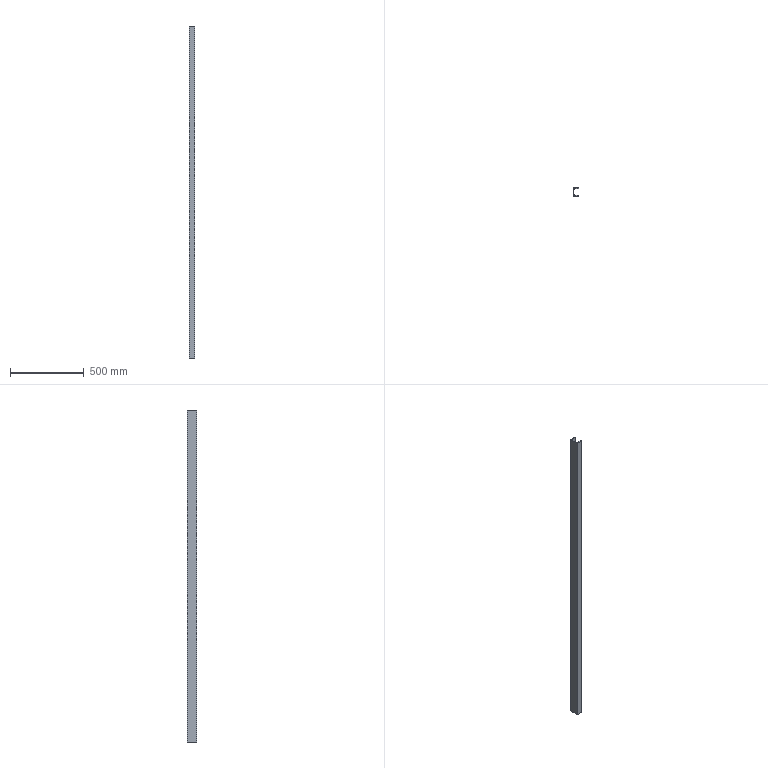Part | STEP file | 750038459 | 1 solid | 14 faces | box 40 x 63 x 2248 mm | volume 1898587 mm3 | plane 10 | cylinder 4 | commonest cylinder face diameters 7.6 x2 15 x2
STEP:
#1=CARTESIAN_POINT('',(0.,0.,2248.));
#2=VERTEX_POINT('',#1);
#3=CARTESIAN_POINT('',(0.,0.,0.));
#4=VERTEX_POINT('',#3);
#5=CARTESIAN_POINT('',(0.,0.,2248.));
#6=DIRECTION('',(0.,0.,-1.));
#7=VECTOR('',#6,1000.);
#8=LINE('',#5,#7);
#9=EDGE_CURVE('',#2,#4,#8,.T.);
#10=ORIENTED_EDGE('',*,*,#9,.F.);
#11=CARTESIAN_POINT('',(0.,63.,2248.));
#12=VERTEX_POINT('',#11);
#13=CARTESIAN_POINT('',(0.,63.,2248.));
#14=DIRECTION('',(0.,-1.,0.));
#15=VECTOR('',#14,1000.);
#16=LINE('',#13,#15);
#17=EDGE_CURVE('',#12,#2,#16,.T.);
#18=ORIENTED_EDGE('',*,*,#17,.F.);
#19=CARTESIAN_POINT('',(0.,63.,0.));
#20=VERTEX_POINT('',#19);
#21=CARTESIAN_POINT('',(0.,63.,2248.));
#22=DIRECTION('',(0.,0.,1.));
#23=VECTOR('',#22,1000.);
#24=LINE('',#21,#23);
#25=EDGE_CURVE('',#20,#12,#24,.T.);
#26=ORIENTED_EDGE('',*,*,#25,.F.);
#27=CARTESIAN_POINT('',(0.,63.,0.));
#28=DIRECTION('',(0.,1.,0.));
#29=VECTOR('',#28,1000.);
#30=LINE('',#27,#29);
#31=EDGE_CURVE('',#4,#20,#30,.T.);
#32=ORIENTED_EDGE('',*,*,#31,.F.);
#33=EDGE_LOOP('',(#10,#18,#26,#32));
#34=FACE_OUTER_BOUND('',#33,.T.);
#35=CARTESIAN_POINT('',(0.,63.,2248.));
#36=DIRECTION('',(1.,0.,0.));
#37=DIRECTION('',(0.,0.,-1.));
#38=AXIS2_PLACEMENT_3D('',#35,#36,#37);
#39=PLANE('',#38);
#40=ADVANCED_FACE('',(#34),#39,.F.);
#41=CARTESIAN_POINT('',(40.,63.,0.));
#42=VERTEX_POINT('',#41);
#43=CARTESIAN_POINT('',(36.2,63.,0.));
#44=DIRECTION('',(-1.,0.,0.));
#45=VECTOR('',#44,1000.);
#46=LINE('',#43,#45);
#47=EDGE_CURVE('',#42,#20,#46,.T.);
#48=ORIENTED_EDGE('',*,*,#47,.F.);
#49=CARTESIAN_POINT('',(40.,60.699,0.));
#50=VERTEX_POINT('',#49);
#51=CARTESIAN_POINT('',(40.,2.301,0.));
#52=DIRECTION('',(0.,1.,0.));
#53=VECTOR('',#52,1000.);
#54=LINE('',#51,#53);
#55=EDGE_CURVE('',#50,#42,#54,.T.);
#56=ORIENTED_EDGE('',*,*,#55,.F.);
#57=CARTESIAN_POINT('',(36.578,56.918,0.));
#58=VERTEX_POINT('',#57);
#59=CARTESIAN_POINT('',(36.2,60.699,0.));
#60=DIRECTION('',(0.,0.,1.));
#61=DIRECTION('',(-1.,0.,0.));
#62=AXIS2_PLACEMENT_3D('',#59,#60,#61);
#63=CIRCLE('',#62,3.8);
#64=EDGE_CURVE('',#58,#50,#63,.T.);
#65=ORIENTED_EDGE('',*,*,#64,.F.);
#66=CARTESIAN_POINT('',(11.554,54.415,0.));
#67=VERTEX_POINT('',#66);
#68=CARTESIAN_POINT('',(11.554,54.415,0.));
#69=DIRECTION('',(0.995,0.0995,0.));
#70=VECTOR('',#69,1000.);
#71=LINE('',#68,#70);
#72=EDGE_CURVE('',#67,#58,#71,.T.);
#73=ORIENTED_EDGE('',*,*,#72,.F.);
#74=CARTESIAN_POINT('',(4.8,46.953,0.));
#75=VERTEX_POINT('',#74);
#76=CARTESIAN_POINT('',(12.3,46.953,0.));
#77=DIRECTION('',(0.,0.,-1.));
#78=DIRECTION('',(-1.,0.,0.));
#79=AXIS2_PLACEMENT_3D('',#76,#77,#78);
#80=CIRCLE('',#79,7.5);
#81=EDGE_CURVE('',#75,#67,#80,.T.);
#82=ORIENTED_EDGE('',*,*,#81,.F.);
#83=CARTESIAN_POINT('',(4.8,16.047,0.));
#84=VERTEX_POINT('',#83);
#85=CARTESIAN_POINT('',(4.8,2.301,0.));
#86=DIRECTION('',(0.,1.,0.));
#87=VECTOR('',#86,1000.);
#88=LINE('',#85,#87);
#89=EDGE_CURVE('',#84,#75,#88,.T.);
#90=ORIENTED_EDGE('',*,*,#89,.F.);
#91=CARTESIAN_POINT('',(11.554,8.585,0.));
#92=VERTEX_POINT('',#91);
#93=CARTESIAN_POINT('',(12.3,16.047,0.));
#94=DIRECTION('',(0.,0.,-1.));
#95=DIRECTION('',(-1.,0.,0.));
#96=AXIS2_PLACEMENT_3D('',#93,#94,#95);
#97=CIRCLE('',#96,7.5);
#98=EDGE_CURVE('',#92,#84,#97,.T.);
#99=ORIENTED_EDGE('',*,*,#98,.F.);
#100=CARTESIAN_POINT('',(36.578,6.082,0.));
#101=VERTEX_POINT('',#100);
#102=CARTESIAN_POINT('',(36.578,6.082,0.));
#103=DIRECTION('',(-0.995,0.0995,0.));
#104=VECTOR('',#103,1000.);
#105=LINE('',#102,#104);
#106=EDGE_CURVE('',#101,#92,#105,.T.);
#107=ORIENTED_EDGE('',*,*,#106,.F.);
#108=CARTESIAN_POINT('',(40.,2.301,0.));
#109=VERTEX_POINT('',#108);
#110=CARTESIAN_POINT('',(36.2,2.301,0.));
#111=DIRECTION('',(0.,0.,1.));
#112=DIRECTION('',(-1.,0.,0.));
#113=AXIS2_PLACEMENT_3D('',#110,#111,#112);
#114=CIRCLE('',#113,3.8);
#115=EDGE_CURVE('',#109,#101,#114,.T.);
#116=ORIENTED_EDGE('',*,*,#115,.F.);
#117=CARTESIAN_POINT('',(40.,0.,0.));
#118=VERTEX_POINT('',#117);
#119=CARTESIAN_POINT('',(40.,2.301,0.));
#120=DIRECTION('',(0.,1.,0.));
#121=VECTOR('',#120,1000.);
#122=LINE('',#119,#121);
#123=EDGE_CURVE('',#118,#109,#122,.T.);
#124=ORIENTED_EDGE('',*,*,#123,.F.);
#125=CARTESIAN_POINT('',(36.2,0.,0.));
#126=DIRECTION('',(1.,0.,0.));
#127=VECTOR('',#126,1000.);
#128=LINE('',#125,#127);
#129=EDGE_CURVE('',#4,#118,#128,.T.);
#130=ORIENTED_EDGE('',*,*,#129,.F.);
#131=ORIENTED_EDGE('',*,*,#31,.T.);
#132=EDGE_LOOP('',(#48,#56,#65,#73,#82,#90,#99,#107,#116,#124,#130,#131));
#133=FACE_OUTER_BOUND('',#132,.T.);
#134=CARTESIAN_POINT('',(36.2,2.301,0.));
#135=DIRECTION('',(0.,0.,1.));
#136=DIRECTION('',(1.,0.,0.));
#137=AXIS2_PLACEMENT_3D('',#134,#135,#136);
#138=PLANE('',#137);
#139=ADVANCED_FACE('',(#133),#138,.F.);
#140=CARTESIAN_POINT('',(40.,0.,2248.));
#141=VERTEX_POINT('',#140);
#142=CARTESIAN_POINT('',(40.,0.,2248.));
#143=DIRECTION('',(0.,0.,-1.));
#144=VECTOR('',#143,1000.);
#145=LINE('',#142,#144);
#146=EDGE_CURVE('',#141,#118,#145,.T.);
#147=ORIENTED_EDGE('',*,*,#146,.F.);
#148=CARTESIAN_POINT('',(0.,0.,2248.));
#149=DIRECTION('',(1.,0.,0.));
#150=VECTOR('',#149,1000.);
#151=LINE('',#148,#150);
#152=EDGE_CURVE('',#2,#141,#151,.T.);
#153=ORIENTED_EDGE('',*,*,#152,.F.);
#154=ORIENTED_EDGE('',*,*,#9,.T.);
#155=ORIENTED_EDGE('',*,*,#129,.T.);
#156=EDGE_LOOP('',(#147,#153,#154,#155));
#157=FACE_OUTER_BOUND('',#156,.T.);
#158=CARTESIAN_POINT('',(0.,0.,2248.));
#159=DIRECTION('',(0.,1.,0.));
#160=DIRECTION('',(0.,0.,1.));
#161=AXIS2_PLACEMENT_3D('',#158,#159,#160);
#162=PLANE('',#161);
#163=ADVANCED_FACE('',(#157),#162,.F.);
#164=CARTESIAN_POINT('',(40.,60.699,2248.));
#165=VERTEX_POINT('',#164);
#166=CARTESIAN_POINT('',(40.,63.,2248.));
#167=VERTEX_POINT('',#166);
#168=CARTESIAN_POINT('',(40.,2.301,2248.));
#169=DIRECTION('',(0.,1.,0.));
#170=VECTOR('',#169,1000.);
#171=LINE('',#168,#170);
#172=EDGE_CURVE('',#165,#167,#171,.T.);
#173=ORIENTED_EDGE('',*,*,#172,.T.);
#174=CARTESIAN_POINT('',(36.2,63.,2248.));
#175=DIRECTION('',(-1.,0.,0.));
#176=VECTOR('',#175,1000.);
#177=LINE('',#174,#176);
#178=EDGE_CURVE('',#167,#12,#177,.T.);
#179=ORIENTED_EDGE('',*,*,#178,.T.);
#180=ORIENTED_EDGE('',*,*,#17,.T.);
#181=ORIENTED_EDGE('',*,*,#152,.T.);
#182=CARTESIAN_POINT('',(40.,2.301,2248.));
#183=VERTEX_POINT('',#182);
#184=CARTESIAN_POINT('',(40.,2.301,2248.));
#185=DIRECTION('',(0.,1.,0.));
#186=VECTOR('',#185,1000.);
#187=LINE('',#184,#186);
#188=EDGE_CURVE('',#141,#183,#187,.T.);
#189=ORIENTED_EDGE('',*,*,#188,.T.);
#190=CARTESIAN_POINT('',(36.578,6.082,2248.));
#191=VERTEX_POINT('',#190);
#192=CARTESIAN_POINT('',(36.2,2.301,2248.));
#193=DIRECTION('',(0.,0.,1.));
#194=DIRECTION('',(-1.,0.,0.));
#195=AXIS2_PLACEMENT_3D('',#192,#193,#194);
#196=CIRCLE('',#195,3.8);
#197=EDGE_CURVE('',#183,#191,#196,.T.);
#198=ORIENTED_EDGE('',*,*,#197,.T.);
#199=CARTESIAN_POINT('',(11.554,8.585,2248.));
#200=VERTEX_POINT('',#199);
#201=CARTESIAN_POINT('',(36.578,6.082,2248.));
#202=DIRECTION('',(-0.995,0.0995,0.));
#203=VECTOR('',#202,1000.);
#204=LINE('',#201,#203);
#205=EDGE_CURVE('',#191,#200,#204,.T.);
#206=ORIENTED_EDGE('',*,*,#205,.T.);
#207=CARTESIAN_POINT('',(4.8,16.047,2248.));
#208=VERTEX_POINT('',#207);
#209=CARTESIAN_POINT('',(12.3,16.047,2248.));
#210=DIRECTION('',(0.,0.,-1.));
#211=DIRECTION('',(-1.,0.,0.));
#212=AXIS2_PLACEMENT_3D('',#209,#210,#211);
#213=CIRCLE('',#212,7.5);
#214=EDGE_CURVE('',#200,#208,#213,.T.);
#215=ORIENTED_EDGE('',*,*,#214,.T.);
#216=CARTESIAN_POINT('',(4.8,46.953,2248.));
#217=VERTEX_POINT('',#216);
#218=CARTESIAN_POINT('',(4.8,2.301,2248.));
#219=DIRECTION('',(0.,1.,0.));
#220=VECTOR('',#219,1000.);
#221=LINE('',#218,#220);
#222=EDGE_CURVE('',#208,#217,#221,.T.);
#223=ORIENTED_EDGE('',*,*,#222,.T.);
#224=CARTESIAN_POINT('',(11.554,54.415,2248.));
#225=VERTEX_POINT('',#224);
#226=CARTESIAN_POINT('',(12.3,46.953,2248.));
#227=DIRECTION('',(0.,0.,-1.));
#228=DIRECTION('',(-1.,0.,0.));
#229=AXIS2_PLACEMENT_3D('',#226,#227,#228);
#230=CIRCLE('',#229,7.5);
#231=EDGE_CURVE('',#217,#225,#230,.T.);
#232=ORIENTED_EDGE('',*,*,#231,.T.);
#233=CARTESIAN_POINT('',(36.578,56.918,2248.));
#234=VERTEX_POINT('',#233);
#235=CARTESIAN_POINT('',(11.554,54.415,2248.));
#236=DIRECTION('',(0.995,0.0995,0.));
#237=VECTOR('',#236,1000.);
#238=LINE('',#235,#237);
#239=EDGE_CURVE('',#225,#234,#238,.T.);
#240=ORIENTED_EDGE('',*,*,#239,.T.);
#241=CARTESIAN_POINT('',(36.2,60.699,2248.));
#242=DIRECTION('',(0.,0.,1.));
#243=DIRECTION('',(-1.,0.,0.));
#244=AXIS2_PLACEMENT_3D('',#241,#242,#243);
#245=CIRCLE('',#244,3.8);
#246=EDGE_CURVE('',#234,#165,#245,.T.);
#247=ORIENTED_EDGE('',*,*,#246,.T.);
#248=EDGE_LOOP('',(#173,#179,#180,#181,#189,#198,#206,#215,#223,#232,#240,#247));
#249=FACE_OUTER_BOUND('',#248,.T.);
#250=CARTESIAN_POINT('',(36.2,2.301,2248.));
#251=DIRECTION('',(0.,0.,1.));
#252=DIRECTION('',(1.,0.,0.));
#253=AXIS2_PLACEMENT_3D('',#250,#251,#252);
#254=PLANE('',#253);
#255=ADVANCED_FACE('',(#249),#254,.T.);
#256=ORIENTED_EDGE('',*,*,#25,.T.);
#257=ORIENTED_EDGE('',*,*,#178,.F.);
#258=CARTESIAN_POINT('',(40.,63.,2248.));
#259=DIRECTION('',(0.,0.,1.));
#260=VECTOR('',#259,1000.);
#261=LINE('',#258,#260);
#262=EDGE_CURVE('',#42,#167,#261,.T.);
#263=ORIENTED_EDGE('',*,*,#262,.F.);
#264=ORIENTED_EDGE('',*,*,#47,.T.);
#265=EDGE_LOOP('',(#256,#257,#263,#264));
#266=FACE_OUTER_BOUND('',#265,.T.);
#267=CARTESIAN_POINT('',(40.,63.,2248.));
#268=DIRECTION('',(0.,-1.,0.));
#269=DIRECTION('',(0.,0.,-1.));
#270=AXIS2_PLACEMENT_3D('',#267,#268,#269);
#271=PLANE('',#270);
#272=ADVANCED_FACE('',(#266),#271,.F.);
#273=ORIENTED_EDGE('',*,*,#262,.T.);
#274=ORIENTED_EDGE('',*,*,#172,.F.);
#275=CARTESIAN_POINT('',(40.,60.699,2248.));
#276=DIRECTION('',(0.,0.,1.));
#277=VECTOR('',#276,1000.);
#278=LINE('',#275,#277);
#279=EDGE_CURVE('',#50,#165,#278,.T.);
#280=ORIENTED_EDGE('',*,*,#279,.F.);
#281=ORIENTED_EDGE('',*,*,#55,.T.);
#282=EDGE_LOOP('',(#273,#274,#280,#281));
#283=FACE_OUTER_BOUND('',#282,.T.);
#284=CARTESIAN_POINT('',(40.,60.699,2248.));
#285=DIRECTION('',(-1.,0.,0.));
#286=DIRECTION('',(0.,-1.,0.));
#287=AXIS2_PLACEMENT_3D('',#284,#285,#286);
#288=PLANE('',#287);
#289=ADVANCED_FACE('',(#283),#288,.F.);
#290=ORIENTED_EDGE('',*,*,#246,.F.);
#291=CARTESIAN_POINT('',(36.578,56.918,2248.));
#292=DIRECTION('',(0.,0.,-1.));
#293=VECTOR('',#292,1000.);
#294=LINE('',#291,#293);
#295=EDGE_CURVE('',#234,#58,#294,.T.);
#296=ORIENTED_EDGE('',*,*,#295,.T.);
#297=ORIENTED_EDGE('',*,*,#64,.T.);
#298=ORIENTED_EDGE('',*,*,#279,.T.);
#299=EDGE_LOOP('',(#290,#296,#297,#298));
#300=FACE_OUTER_BOUND('',#299,.T.);
#301=CARTESIAN_POINT('',(36.2,60.699,2248.));
#302=DIRECTION('',(0.,0.,-1.));
#303=DIRECTION('',(-1.,0.,0.));
#304=AXIS2_PLACEMENT_3D('',#301,#302,#303);
#305=CYLINDRICAL_SURFACE('',#304,3.8);
#306=ADVANCED_FACE('',(#300),#305,.T.);
#307=ORIENTED_EDGE('',*,*,#295,.F.);
#308=ORIENTED_EDGE('',*,*,#239,.F.);
#309=CARTESIAN_POINT('',(11.554,54.415,2248.));
#310=DIRECTION('',(0.,0.,1.));
#311=VECTOR('',#310,1000.);
#312=LINE('',#309,#311);
#313=EDGE_CURVE('',#67,#225,#312,.T.);
#314=ORIENTED_EDGE('',*,*,#313,.F.);
#315=ORIENTED_EDGE('',*,*,#72,.T.);
#316=EDGE_LOOP('',(#307,#308,#314,#315));
#317=FACE_OUTER_BOUND('',#316,.T.);
#318=CARTESIAN_POINT('',(11.554,54.415,2248.));
#319=DIRECTION('',(-0.0995,0.995,0.));
#320=DIRECTION('',(-0.995,-0.0995,0.));
#321=AXIS2_PLACEMENT_3D('',#318,#319,#320);
#322=PLANE('',#321);
#323=ADVANCED_FACE('',(#317),#322,.F.);
#324=ORIENTED_EDGE('',*,*,#313,.T.);
#325=ORIENTED_EDGE('',*,*,#231,.F.);
#326=CARTESIAN_POINT('',(4.8,46.953,2248.));
#327=DIRECTION('',(0.,0.,1.));
#328=VECTOR('',#327,1000.);
#329=LINE('',#326,#328);
#330=EDGE_CURVE('',#75,#217,#329,.T.);
#331=ORIENTED_EDGE('',*,*,#330,.F.);
#332=ORIENTED_EDGE('',*,*,#81,.T.);
#333=EDGE_LOOP('',(#324,#325,#331,#332));
#334=FACE_OUTER_BOUND('',#333,.T.);
#335=CARTESIAN_POINT('',(12.3,46.953,2248.));
#336=DIRECTION('',(0.,0.,-1.));
#337=DIRECTION('',(-1.,0.,0.));
#338=AXIS2_PLACEMENT_3D('',#335,#336,#337);
#339=CYLINDRICAL_SURFACE('',#338,7.5);
#340=ADVANCED_FACE('',(#334),#339,.F.);
#341=ORIENTED_EDGE('',*,*,#330,.T.);
#342=ORIENTED_EDGE('',*,*,#222,.F.);
#343=CARTESIAN_POINT('',(4.8,16.047,2248.));
#344=DIRECTION('',(0.,0.,1.));
#345=VECTOR('',#344,1000.);
#346=LINE('',#343,#345);
#347=EDGE_CURVE('',#84,#208,#346,.T.);
#348=ORIENTED_EDGE('',*,*,#347,.F.);
#349=ORIENTED_EDGE('',*,*,#89,.T.);
#350=EDGE_LOOP('',(#341,#342,#348,#349));
#351=FACE_OUTER_BOUND('',#350,.T.);
#352=CARTESIAN_POINT('',(4.8,16.047,2248.));
#353=DIRECTION('',(-1.,0.,0.));
#354=DIRECTION('',(0.,-1.,0.));
#355=AXIS2_PLACEMENT_3D('',#352,#353,#354);
#356=PLANE('',#355);
#357=ADVANCED_FACE('',(#351),#356,.F.);
#358=ORIENTED_EDGE('',*,*,#347,.T.);
#359=ORIENTED_EDGE('',*,*,#214,.F.);
#360=CARTESIAN_POINT('',(11.554,8.585,2248.));
#361=DIRECTION('',(0.,0.,1.));
#362=VECTOR('',#361,1000.);
#363=LINE('',#360,#362);
#364=EDGE_CURVE('',#92,#200,#363,.T.);
#365=ORIENTED_EDGE('',*,*,#364,.F.);
#366=ORIENTED_EDGE('',*,*,#98,.T.);
#367=EDGE_LOOP('',(#358,#359,#365,#366));
#368=FACE_OUTER_BOUND('',#367,.T.);
#369=CARTESIAN_POINT('',(12.3,16.047,2248.));
#370=DIRECTION('',(0.,0.,-1.));
#371=DIRECTION('',(-1.,0.,0.));
#372=AXIS2_PLACEMENT_3D('',#369,#370,#371);
#373=CYLINDRICAL_SURFACE('',#372,7.5);
#374=ADVANCED_FACE('',(#368),#373,.F.);
#375=ORIENTED_EDGE('',*,*,#364,.T.);
#376=ORIENTED_EDGE('',*,*,#205,.F.);
#377=CARTESIAN_POINT('',(36.578,6.082,2248.));
#378=DIRECTION('',(0.,0.,1.));
#379=VECTOR('',#378,1000.);
#380=LINE('',#377,#379);
#381=EDGE_CURVE('',#101,#191,#380,.T.);
#382=ORIENTED_EDGE('',*,*,#381,.F.);
#383=ORIENTED_EDGE('',*,*,#106,.T.);
#384=EDGE_LOOP('',(#375,#376,#382,#383));
#385=FACE_OUTER_BOUND('',#384,.T.);
#386=CARTESIAN_POINT('',(36.578,6.082,2248.));
#387=DIRECTION('',(-0.0995,-0.995,0.));
#388=DIRECTION('',(0.995,-0.0995,0.));
#389=AXIS2_PLACEMENT_3D('',#386,#387,#388);
#390=PLANE('',#389);
#391=ADVANCED_FACE('',(#385),#390,.F.);
#392=ORIENTED_EDGE('',*,*,#197,.F.);
#393=CARTESIAN_POINT('',(40.,2.301,2248.));
#394=DIRECTION('',(0.,0.,-1.));
#395=VECTOR('',#394,1000.);
#396=LINE('',#393,#395);
#397=EDGE_CURVE('',#183,#109,#396,.T.);
#398=ORIENTED_EDGE('',*,*,#397,.T.);
#399=ORIENTED_EDGE('',*,*,#115,.T.);
#400=ORIENTED_EDGE('',*,*,#381,.T.);
#401=EDGE_LOOP('',(#392,#398,#399,#400));
#402=FACE_OUTER_BOUND('',#401,.T.);
#403=CARTESIAN_POINT('',(36.2,2.301,2248.));
#404=DIRECTION('',(0.,0.,-1.));
#405=DIRECTION('',(-1.,0.,0.));
#406=AXIS2_PLACEMENT_3D('',#403,#404,#405);
#407=CYLINDRICAL_SURFACE('',#406,3.8);
#408=ADVANCED_FACE('',(#402),#407,.T.);
#409=ORIENTED_EDGE('',*,*,#397,.F.);
#410=ORIENTED_EDGE('',*,*,#188,.F.);
#411=ORIENTED_EDGE('',*,*,#146,.T.);
#412=ORIENTED_EDGE('',*,*,#123,.T.);
#413=EDGE_LOOP('',(#409,#410,#411,#412));
#414=FACE_OUTER_BOUND('',#413,.T.);
#415=CARTESIAN_POINT('',(40.,0.,2248.));
#416=DIRECTION('',(-1.,0.,0.));
#417=DIRECTION('',(0.,0.,1.));
#418=AXIS2_PLACEMENT_3D('',#415,#416,#417);
#419=PLANE('',#418);
#420=ADVANCED_FACE('',(#414),#419,.F.);
#421=CLOSED_SHELL('',(#40,#139,#163,#255,#272,#289,#306,#323,#340,#357,#374,#391,#408,#420));
#422=MANIFOLD_SOLID_BREP('',#421);
#423=CARTESIAN_POINT('',(0.,0.,0.));
#424=DIRECTION('',(0.,0.,1.));
#425=DIRECTION('',(1.,0.,0.));
#426=AXIS2_PLACEMENT_3D('',#423,#424,#425);
#427=(LENGTH_UNIT()NAMED_UNIT(*)SI_UNIT(.MILLI.,.METRE.));
#428=UNCERTAINTY_MEASURE_WITH_UNIT(LENGTH_MEASURE(0.00001),#427,'','');
#429=(NAMED_UNIT(*)PLANE_ANGLE_UNIT()SI_UNIT($,.RADIAN.));
#430=(NAMED_UNIT(*)SI_UNIT($,.STERADIAN.)SOLID_ANGLE_UNIT());
#431=(GEOMETRIC_REPRESENTATION_CONTEXT(3)GLOBAL_UNCERTAINTY_ASSIGNED_CONTEXT((#428))GLOBAL_UNIT_ASSIGNED_CONTEXT((#427,#429,#430))REPRESENTATION_CONTEXT('',''));
#432=ADVANCED_BREP_SHAPE_REPRESENTATION('',(#422,#426),#431);